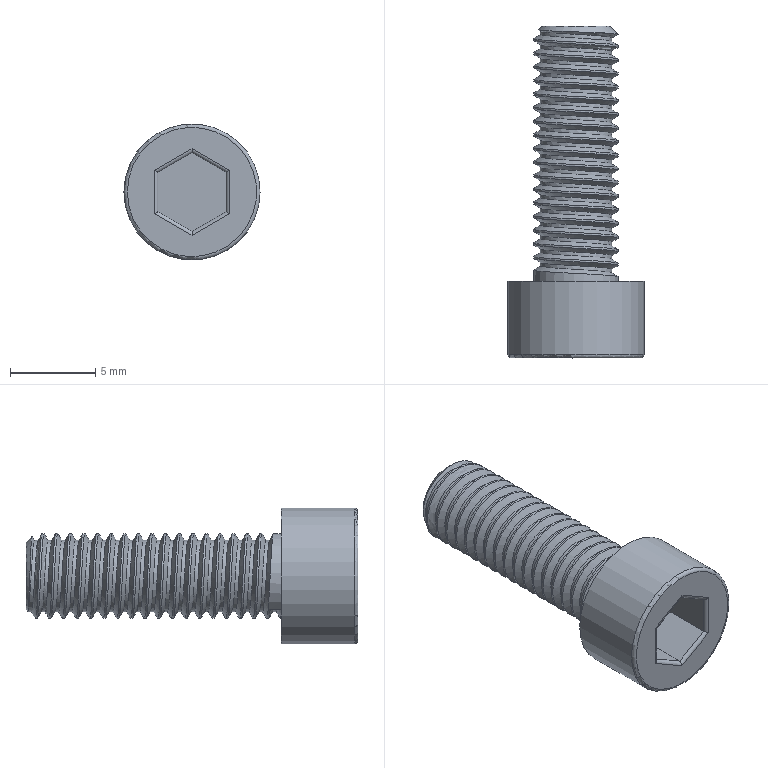Part | STEP file | Tube feed_id982_x_t | 1 solid | 27 faces | box 8 x 19.5 x 8 mm | volume 422.965 mm3 | plane 12 | cylinder 9 | spline 3 | cone 2 | torus 1 | commonest cylinder face diameters 0.4 x6 4.2 x1 5 x1 8 x1